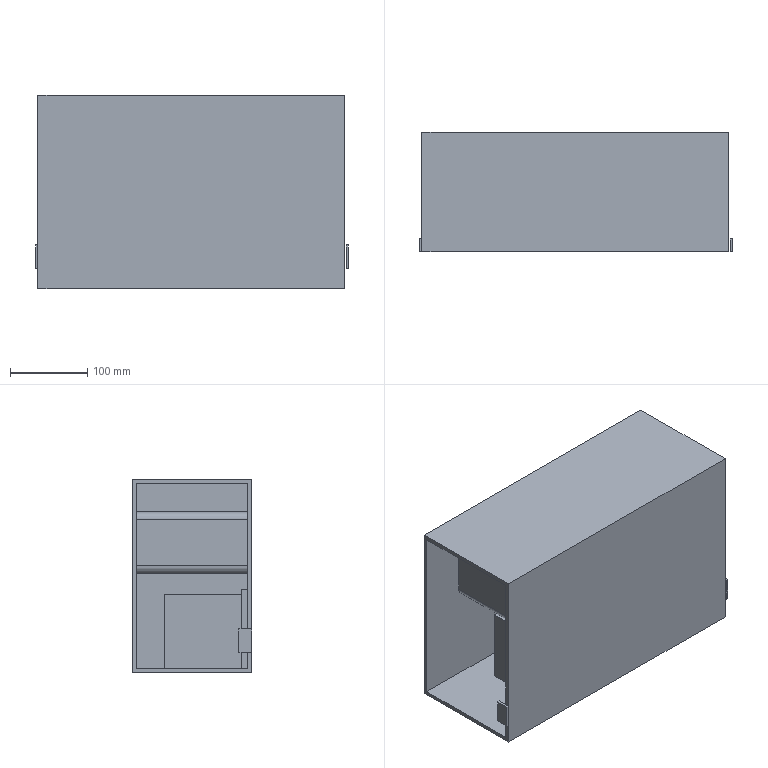Part | SolidWorks | features BaseBody 5 | 5 solids | 51 faces | box 406 x 155 x 251.525 mm | volume 5535552 mm3 | plane 43 | cylinder 8 | commonest cylinder face diameters 20 x8
STEP:
#1=CARTESIAN_POINT('',(141.539,102.72,635.851));
#2=VERTEX_POINT('',#1);
#3=CARTESIAN_POINT('',(271.539,102.72,635.851));
#4=VERTEX_POINT('',#3);
#5=CARTESIAN_POINT('',(0.,102.72,635.851));
#6=DIRECTION('',(1.,0.,0.));
#7=VECTOR('',#6,1000.);
#8=LINE('',#5,#7);
#9=EDGE_CURVE('',#2,#4,#8,.T.);
#10=ORIENTED_EDGE('',*,*,#9,.T.);
#11=CARTESIAN_POINT('',(271.539,102.72,532.815));
#12=VERTEX_POINT('',#11);
#13=CARTESIAN_POINT('',(271.539,102.72,-148.475));
#14=DIRECTION('',(0.,0.,-1.));
#15=VECTOR('',#14,1000.);
#16=LINE('',#13,#15);
#17=EDGE_CURVE('',#4,#12,#16,.T.);
#18=ORIENTED_EDGE('',*,*,#17,.T.);
#19=CARTESIAN_POINT('',(141.539,102.72,532.815));
#20=VERTEX_POINT('',#19);
#21=CARTESIAN_POINT('',(0.,102.72,532.815));
#22=DIRECTION('',(-1.,0.,0.));
#23=VECTOR('',#22,1000.);
#24=LINE('',#21,#23);
#25=EDGE_CURVE('',#12,#20,#24,.T.);
#26=ORIENTED_EDGE('',*,*,#25,.T.);
#27=CARTESIAN_POINT('',(141.539,102.72,-148.475));
#28=DIRECTION('',(0.,0.,1.));
#29=VECTOR('',#28,1000.);
#30=LINE('',#27,#29);
#31=EDGE_CURVE('',#20,#2,#30,.T.);
#32=ORIENTED_EDGE('',*,*,#31,.T.);
#33=EDGE_LOOP('',(#10,#18,#26,#32));
#34=FACE_OUTER_BOUND('',#33,.T.);
#35=CARTESIAN_POINT('',(0.,102.72,-148.475));
#36=DIRECTION('',(0.,1.,0.));
#37=DIRECTION('',(0.,0.,1.));
#38=AXIS2_PLACEMENT_3D('',#35,#36,#37);
#39=PLANE('',#38);
#40=ADVANCED_FACE('',(#34),#39,.T.);
#41=CARTESIAN_POINT('',(271.539,94.72,532.815));
#42=VERTEX_POINT('',#41);
#43=CARTESIAN_POINT('',(271.539,102.72,532.815));
#44=DIRECTION('',(0.,-1.,0.));
#45=VECTOR('',#44,1000.);
#46=LINE('',#43,#45);
#47=EDGE_CURVE('',#12,#42,#46,.T.);
#48=ORIENTED_EDGE('',*,*,#47,.F.);
#49=ORIENTED_EDGE('',*,*,#17,.F.);
#50=CARTESIAN_POINT('',(271.539,94.72,635.851));
#51=VERTEX_POINT('',#50);
#52=CARTESIAN_POINT('',(271.539,102.72,635.851));
#53=DIRECTION('',(0.,1.,0.));
#54=VECTOR('',#53,1000.);
#55=LINE('',#52,#54);
#56=EDGE_CURVE('',#51,#4,#55,.T.);
#57=ORIENTED_EDGE('',*,*,#56,.F.);
#58=CARTESIAN_POINT('',(271.539,94.72,475.851));
#59=DIRECTION('',(0.,0.,1.));
#60=VECTOR('',#59,1000.);
#61=LINE('',#58,#60);
#62=EDGE_CURVE('',#42,#51,#61,.T.);
#63=ORIENTED_EDGE('',*,*,#62,.F.);
#64=EDGE_LOOP('',(#48,#49,#57,#63));
#65=FACE_OUTER_BOUND('',#64,.T.);
#66=CARTESIAN_POINT('',(271.539,102.72,475.851));
#67=DIRECTION('',(-1.,0.,0.));
#68=DIRECTION('',(0.,0.,1.));
#69=AXIS2_PLACEMENT_3D('',#66,#67,#68);
#70=PLANE('',#69);
#71=ADVANCED_FACE('',(#65),#70,.F.);
#72=ORIENTED_EDGE('',*,*,#56,.T.);
#73=ORIENTED_EDGE('',*,*,#9,.F.);
#74=CARTESIAN_POINT('',(141.539,94.72,635.851));
#75=VERTEX_POINT('',#74);
#76=CARTESIAN_POINT('',(141.539,102.72,635.851));
#77=DIRECTION('',(0.,1.,0.));
#78=VECTOR('',#77,1000.);
#79=LINE('',#76,#78);
#80=EDGE_CURVE('',#75,#2,#79,.T.);
#81=ORIENTED_EDGE('',*,*,#80,.F.);
#82=CARTESIAN_POINT('',(141.539,94.72,635.851));
#83=DIRECTION('',(-1.,0.,0.));
#84=VECTOR('',#83,1000.);
#85=LINE('',#82,#84);
#86=EDGE_CURVE('',#51,#75,#85,.T.);
#87=ORIENTED_EDGE('',*,*,#86,.F.);
#88=EDGE_LOOP('',(#72,#73,#81,#87));
#89=FACE_OUTER_BOUND('',#88,.T.);
#90=CARTESIAN_POINT('',(141.539,102.72,635.851));
#91=DIRECTION('',(0.,0.,-1.));
#92=DIRECTION('',(-1.,0.,0.));
#93=AXIS2_PLACEMENT_3D('',#90,#91,#92);
#94=PLANE('',#93);
#95=ADVANCED_FACE('',(#89),#94,.F.);
#96=CARTESIAN_POINT('',(141.539,94.72,532.815));
#97=VERTEX_POINT('',#96);
#98=CARTESIAN_POINT('',(141.539,102.72,532.815));
#99=DIRECTION('',(0.,1.,0.));
#100=VECTOR('',#99,1000.);
#101=LINE('',#98,#100);
#102=EDGE_CURVE('',#97,#20,#101,.T.);
#103=ORIENTED_EDGE('',*,*,#102,.F.);
#104=CARTESIAN_POINT('',(141.539,94.72,475.851));
#105=DIRECTION('',(0.,0.,-1.));
#106=VECTOR('',#105,1000.);
#107=LINE('',#104,#106);
#108=EDGE_CURVE('',#75,#97,#107,.T.);
#109=ORIENTED_EDGE('',*,*,#108,.F.);
#110=ORIENTED_EDGE('',*,*,#80,.T.);
#111=ORIENTED_EDGE('',*,*,#31,.F.);
#112=EDGE_LOOP('',(#103,#109,#110,#111));
#113=FACE_OUTER_BOUND('',#112,.T.);
#114=CARTESIAN_POINT('',(141.539,102.72,475.851));
#115=DIRECTION('',(1.,0.,0.));
#116=DIRECTION('',(0.,0.,-1.));
#117=AXIS2_PLACEMENT_3D('',#114,#115,#116);
#118=PLANE('',#117);
#119=ADVANCED_FACE('',(#113),#118,.F.);
#120=ORIENTED_EDGE('',*,*,#47,.T.);
#121=CARTESIAN_POINT('',(460.124,94.72,532.815));
#122=DIRECTION('',(1.,0.,0.));
#123=VECTOR('',#122,1000.);
#124=LINE('',#121,#123);
#125=EDGE_CURVE('',#97,#42,#124,.T.);
#126=ORIENTED_EDGE('',*,*,#125,.F.);
#127=ORIENTED_EDGE('',*,*,#102,.T.);
#128=ORIENTED_EDGE('',*,*,#25,.F.);
#129=EDGE_LOOP('',(#120,#126,#127,#128));
#130=FACE_OUTER_BOUND('',#129,.T.);
#131=CARTESIAN_POINT('',(460.124,-110.28,532.815));
#132=DIRECTION('',(0.,0.,1.));
#133=DIRECTION('',(1.,0.,0.));
#134=AXIS2_PLACEMENT_3D('',#131,#132,#133);
#135=PLANE('',#134);
#136=ADVANCED_FACE('',(#130),#135,.F.);
#137=ORIENTED_EDGE('',*,*,#125,.T.);
#138=ORIENTED_EDGE('',*,*,#62,.T.);
#139=ORIENTED_EDGE('',*,*,#86,.T.);
#140=ORIENTED_EDGE('',*,*,#108,.T.);
#141=EDGE_LOOP('',(#137,#138,#139,#140));
#142=FACE_OUTER_BOUND('',#141,.T.);
#143=CARTESIAN_POINT('',(0.,94.72,-148.475));
#144=DIRECTION('',(0.,1.,0.));
#145=DIRECTION('',(0.,0.,1.));
#146=AXIS2_PLACEMENT_3D('',#143,#144,#145);
#147=PLANE('',#146);
#148=ADVANCED_FACE('',(#142),#147,.F.);
#149=CLOSED_SHELL('',(#40,#71,#95,#119,#136,#148));
#150=MANIFOLD_SOLID_BREP('',#149);
#151=CARTESIAN_POINT('',(460.124,89.72,584.76));
#152=VERTEX_POINT('',#151);
#153=CARTESIAN_POINT('',(460.124,89.72,554.76));
#154=VERTEX_POINT('',#153);
#155=CARTESIAN_POINT('',(460.124,89.72,584.76));
#156=DIRECTION('',(0.,0.,-1.));
#157=VECTOR('',#156,1000.);
#158=LINE('',#155,#157);
#159=EDGE_CURVE('',#152,#154,#158,.T.);
#160=ORIENTED_EDGE('',*,*,#159,.F.);
#161=CARTESIAN_POINT('',(460.124,106.359,584.76));
#162=VERTEX_POINT('',#161);
#163=CARTESIAN_POINT('',(460.124,72.987,584.76));
#164=DIRECTION('',(0.,-1.,0.));
#165=VECTOR('',#164,1000.);
#166=LINE('',#163,#165);
#167=EDGE_CURVE('',#162,#152,#166,.T.);
#168=ORIENTED_EDGE('',*,*,#167,.F.);
#169=CARTESIAN_POINT('',(460.124,106.359,554.76));
#170=VERTEX_POINT('',#169);
#171=CARTESIAN_POINT('',(460.124,106.359,584.76));
#172=DIRECTION('',(0.,0.,1.));
#173=VECTOR('',#172,1000.);
#174=LINE('',#171,#173);
#175=EDGE_CURVE('',#170,#162,#174,.T.);
#176=ORIENTED_EDGE('',*,*,#175,.F.);
#177=CARTESIAN_POINT('',(460.124,72.987,554.76));
#178=DIRECTION('',(0.,1.,0.));
#179=VECTOR('',#178,1000.);
#180=LINE('',#177,#179);
#181=EDGE_CURVE('',#154,#170,#180,.T.);
#182=ORIENTED_EDGE('',*,*,#181,.F.);
#183=EDGE_LOOP('',(#160,#168,#176,#182));
#184=FACE_OUTER_BOUND('',#183,.T.);
#185=CARTESIAN_POINT('',(460.124,72.987,584.76));
#186=DIRECTION('',(1.,0.,0.));
#187=DIRECTION('',(0.,0.,-1.));
#188=AXIS2_PLACEMENT_3D('',#185,#186,#187);
#189=PLANE('',#188);
#190=ADVANCED_FACE('',(#184),#189,.F.);
#191=CARTESIAN_POINT('',(463.124,106.359,554.76));
#192=VERTEX_POINT('',#191);
#193=CARTESIAN_POINT('',(260.124,106.359,554.76));
#194=DIRECTION('',(1.,0.,0.));
#195=VECTOR('',#194,1000.);
#196=LINE('',#193,#195);
#197=EDGE_CURVE('',#170,#192,#196,.T.);
#198=ORIENTED_EDGE('',*,*,#197,.T.);
#199=CARTESIAN_POINT('',(463.124,89.72,554.76));
#200=VERTEX_POINT('',#199);
#201=CARTESIAN_POINT('',(463.124,59.72,554.76));
#202=DIRECTION('',(0.,-1.,0.));
#203=VECTOR('',#202,1000.);
#204=LINE('',#201,#203);
#205=EDGE_CURVE('',#192,#200,#204,.T.);
#206=ORIENTED_EDGE('',*,*,#205,.T.);
#207=CARTESIAN_POINT('',(260.124,89.72,554.76));
#208=DIRECTION('',(-1.,0.,0.));
#209=VECTOR('',#208,1000.);
#210=LINE('',#207,#209);
#211=EDGE_CURVE('',#200,#154,#210,.T.);
#212=ORIENTED_EDGE('',*,*,#211,.T.);
#213=ORIENTED_EDGE('',*,*,#181,.T.);
#214=EDGE_LOOP('',(#198,#206,#212,#213));
#215=FACE_OUTER_BOUND('',#214,.T.);
#216=CARTESIAN_POINT('',(260.124,59.72,554.76));
#217=DIRECTION('',(0.,0.,-1.));
#218=DIRECTION('',(-1.,0.,0.));
#219=AXIS2_PLACEMENT_3D('',#216,#217,#218);
#220=PLANE('',#219);
#221=ADVANCED_FACE('',(#215),#220,.T.);
#222=ORIENTED_EDGE('',*,*,#211,.F.);
#223=CARTESIAN_POINT('',(463.124,89.72,584.76));
#224=VERTEX_POINT('',#223);
#225=CARTESIAN_POINT('',(463.124,89.72,0.));
#226=DIRECTION('',(0.,0.,-1.));
#227=VECTOR('',#226,1000.);
#228=LINE('',#225,#227);
#229=EDGE_CURVE('',#224,#200,#228,.T.);
#230=ORIENTED_EDGE('',*,*,#229,.F.);
#231=CARTESIAN_POINT('',(0.,89.72,584.76));
#232=DIRECTION('',(1.,0.,0.));
#233=VECTOR('',#232,1000.);
#234=LINE('',#231,#233);
#235=EDGE_CURVE('',#152,#224,#234,.T.);
#236=ORIENTED_EDGE('',*,*,#235,.F.);
#237=ORIENTED_EDGE('',*,*,#159,.T.);
#238=EDGE_LOOP('',(#222,#230,#236,#237));
#239=FACE_OUTER_BOUND('',#238,.T.);
#240=CARTESIAN_POINT('',(0.,89.72,0.));
#241=DIRECTION('',(0.,1.,0.));
#242=DIRECTION('',(0.,0.,1.));
#243=AXIS2_PLACEMENT_3D('',#240,#241,#242);
#244=PLANE('',#243);
#245=ADVANCED_FACE('',(#239),#244,.F.);
#246=ORIENTED_EDGE('',*,*,#235,.T.);
#247=CARTESIAN_POINT('',(463.124,106.359,584.76));
#248=VERTEX_POINT('',#247);
#249=CARTESIAN_POINT('',(463.124,59.72,584.76));
#250=DIRECTION('',(0.,-1.,0.));
#251=VECTOR('',#250,1000.);
#252=LINE('',#249,#251);
#253=EDGE_CURVE('',#248,#224,#252,.T.);
#254=ORIENTED_EDGE('',*,*,#253,.F.);
#255=CARTESIAN_POINT('',(260.124,106.359,584.76));
#256=DIRECTION('',(1.,0.,0.));
#257=VECTOR('',#256,1000.);
#258=LINE('',#255,#257);
#259=EDGE_CURVE('',#162,#248,#258,.T.);
#260=ORIENTED_EDGE('',*,*,#259,.F.);
#261=ORIENTED_EDGE('',*,*,#167,.T.);
#262=EDGE_LOOP('',(#246,#254,#260,#261));
#263=FACE_OUTER_BOUND('',#262,.T.);
#264=CARTESIAN_POINT('',(260.124,59.72,584.76));
#265=DIRECTION('',(0.,0.,-1.));
#266=DIRECTION('',(-1.,0.,0.));
#267=AXIS2_PLACEMENT_3D('',#264,#265,#266);
#268=PLANE('',#267);
#269=ADVANCED_FACE('',(#263),#268,.F.);
#270=ORIENTED_EDGE('',*,*,#175,.T.);
#271=ORIENTED_EDGE('',*,*,#259,.T.);
#272=CARTESIAN_POINT('',(463.124,106.359,584.76));
#273=DIRECTION('',(0.,0.,1.));
#274=VECTOR('',#273,1000.);
#275=LINE('',#272,#274);
#276=EDGE_CURVE('',#192,#248,#275,.T.);
#277=ORIENTED_EDGE('',*,*,#276,.F.);
#278=ORIENTED_EDGE('',*,*,#197,.F.);
#279=EDGE_LOOP('',(#270,#271,#277,#278));
#280=FACE_OUTER_BOUND('',#279,.T.);
#281=CARTESIAN_POINT('',(463.124,106.359,584.76));
#282=DIRECTION('',(0.,-1.,0.));
#283=DIRECTION('',(0.,0.,-1.));
#284=AXIS2_PLACEMENT_3D('',#281,#282,#283);
#285=PLANE('',#284);
#286=ADVANCED_FACE('',(#280),#285,.F.);
#287=ORIENTED_EDGE('',*,*,#229,.T.);
#288=ORIENTED_EDGE('',*,*,#205,.F.);
#289=ORIENTED_EDGE('',*,*,#276,.T.);
#290=ORIENTED_EDGE('',*,*,#253,.T.);
#291=EDGE_LOOP('',(#287,#288,#289,#290));
#292=FACE_OUTER_BOUND('',#291,.T.);
#293=CARTESIAN_POINT('',(463.124,72.987,584.76));
#294=DIRECTION('',(-1.,0.,0.));
#295=DIRECTION('',(0.,0.,1.));
#296=AXIS2_PLACEMENT_3D('',#293,#294,#295);
#297=PLANE('',#296);
#298=ADVANCED_FACE('',(#292),#297,.F.);
#299=CLOSED_SHELL('',(#190,#221,#245,#269,#286,#298));
#300=MANIFOLD_SOLID_BREP('',#299);
#301=CARTESIAN_POINT('',(265.539,102.72,532.815));
#302=VERTEX_POINT('',#301);
#303=CARTESIAN_POINT('',(265.539,202.72,532.815));
#304=VERTEX_POINT('',#303);
#305=CARTESIAN_POINT('',(265.539,-110.28,532.815));
#306=DIRECTION('',(0.,1.,0.));
#307=VECTOR('',#306,1000.);
#308=LINE('',#305,#307);
#309=EDGE_CURVE('',#302,#304,#308,.T.);
#310=ORIENTED_EDGE('',*,*,#309,.F.);
#311=CARTESIAN_POINT('',(147.539,102.72,532.815));
#312=VERTEX_POINT('',#311);
#313=CARTESIAN_POINT('',(460.124,102.72,532.815));
#314=DIRECTION('',(1.,0.,0.));
#315=VECTOR('',#314,1000.);
#316=LINE('',#313,#315);
#317=EDGE_CURVE('',#312,#302,#316,.T.);
#318=ORIENTED_EDGE('',*,*,#317,.F.);
#319=CARTESIAN_POINT('',(147.539,202.72,532.815));
#320=VERTEX_POINT('',#319);
#321=CARTESIAN_POINT('',(147.539,-110.28,532.815));
#322=DIRECTION('',(0.,-1.,0.));
#323=VECTOR('',#322,1000.);
#324=LINE('',#321,#323);
#325=EDGE_CURVE('',#320,#312,#324,.T.);
#326=ORIENTED_EDGE('',*,*,#325,.F.);
#327=CARTESIAN_POINT('',(460.124,202.72,532.815));
#328=DIRECTION('',(-1.,0.,0.));
#329=VECTOR('',#328,1000.);
#330=LINE('',#327,#329);
#331=EDGE_CURVE('',#304,#320,#330,.T.);
#332=ORIENTED_EDGE('',*,*,#331,.F.);
#333=EDGE_LOOP('',(#310,#318,#326,#332));
#334=FACE_OUTER_BOUND('',#333,.T.);
#335=CARTESIAN_POINT('',(460.124,-110.28,532.815));
#336=DIRECTION('',(0.,0.,1.));
#337=DIRECTION('',(1.,0.,0.));
#338=AXIS2_PLACEMENT_3D('',#335,#336,#337);
#339=PLANE('',#338);
#340=ADVANCED_FACE('',(#334),#339,.F.);
#341=CARTESIAN_POINT('',(147.539,202.72,629.851));
#342=VERTEX_POINT('',#341);
#343=CARTESIAN_POINT('',(265.539,202.72,629.851));
#344=VERTEX_POINT('',#343);
#345=CARTESIAN_POINT('',(0.,202.72,629.851));
#346=DIRECTION('',(1.,0.,0.));
#347=VECTOR('',#346,1000.);
#348=LINE('',#345,#347);
#349=EDGE_CURVE('',#342,#344,#348,.T.);
#350=ORIENTED_EDGE('',*,*,#349,.T.);
#351=CARTESIAN_POINT('',(265.539,202.72,-148.475));
#352=DIRECTION('',(0.,0.,-1.));
#353=VECTOR('',#352,1000.);
#354=LINE('',#351,#353);
#355=EDGE_CURVE('',#344,#304,#354,.T.);
#356=ORIENTED_EDGE('',*,*,#355,.T.);
#357=ORIENTED_EDGE('',*,*,#331,.T.);
#358=CARTESIAN_POINT('',(147.539,202.72,-148.475));
#359=DIRECTION('',(0.,0.,1.));
#360=VECTOR('',#359,1000.);
#361=LINE('',#358,#360);
#362=EDGE_CURVE('',#320,#342,#361,.T.);
#363=ORIENTED_EDGE('',*,*,#362,.T.);
#364=EDGE_LOOP('',(#350,#356,#357,#363));
#365=FACE_OUTER_BOUND('',#364,.T.);
#366=CARTESIAN_POINT('',(0.,202.72,-148.475));
#367=DIRECTION('',(0.,1.,0.));
#368=DIRECTION('',(0.,0.,1.));
#369=AXIS2_PLACEMENT_3D('',#366,#367,#368);
#370=PLANE('',#369);
#371=ADVANCED_FACE('',(#365),#370,.T.);
#372=ORIENTED_EDGE('',*,*,#309,.T.);
#373=ORIENTED_EDGE('',*,*,#355,.F.);
#374=CARTESIAN_POINT('',(265.539,102.72,629.851));
#375=VERTEX_POINT('',#374);
#376=CARTESIAN_POINT('',(265.539,202.72,629.851));
#377=DIRECTION('',(0.,1.,0.));
#378=VECTOR('',#377,1000.);
#379=LINE('',#376,#378);
#380=EDGE_CURVE('',#375,#344,#379,.T.);
#381=ORIENTED_EDGE('',*,*,#380,.F.);
#382=CARTESIAN_POINT('',(265.539,102.72,629.851));
#383=DIRECTION('',(0.,0.,1.));
#384=VECTOR('',#383,1000.);
#385=LINE('',#382,#384);
#386=EDGE_CURVE('',#302,#375,#385,.T.);
#387=ORIENTED_EDGE('',*,*,#386,.F.);
#388=EDGE_LOOP('',(#372,#373,#381,#387));
#389=FACE_OUTER_BOUND('',#388,.T.);
#390=CARTESIAN_POINT('',(265.539,202.72,629.851));
#391=DIRECTION('',(-1.,0.,0.));
#392=DIRECTION('',(0.,0.,1.));
#393=AXIS2_PLACEMENT_3D('',#390,#391,#392);
#394=PLANE('',#393);
#395=ADVANCED_FACE('',(#389),#394,.F.);
#396=ORIENTED_EDGE('',*,*,#317,.T.);
#397=ORIENTED_EDGE('',*,*,#386,.T.);
#398=CARTESIAN_POINT('',(147.539,102.72,629.851));
#399=VERTEX_POINT('',#398);
#400=CARTESIAN_POINT('',(0.,102.72,629.851));
#401=DIRECTION('',(1.,0.,0.));
#402=VECTOR('',#401,1000.);
#403=LINE('',#400,#402);
#404=EDGE_CURVE('',#399,#375,#403,.T.);
#405=ORIENTED_EDGE('',*,*,#404,.F.);
#406=CARTESIAN_POINT('',(147.539,102.72,-148.475));
#407=DIRECTION('',(0.,0.,1.));
#408=VECTOR('',#407,1000.);
#409=LINE('',#406,#408);
#410=EDGE_CURVE('',#312,#399,#409,.T.);
#411=ORIENTED_EDGE('',*,*,#410,.F.);
#412=EDGE_LOOP('',(#396,#397,#405,#411));
#413=FACE_OUTER_BOUND('',#412,.T.);
#414=CARTESIAN_POINT('',(0.,102.72,-148.475));
#415=DIRECTION('',(0.,1.,0.));
#416=DIRECTION('',(0.,0.,1.));
#417=AXIS2_PLACEMENT_3D('',#414,#415,#416);
#418=PLANE('',#417);
#419=ADVANCED_FACE('',(#413),#418,.F.);
#420=ORIENTED_EDGE('',*,*,#325,.T.);
#421=ORIENTED_EDGE('',*,*,#410,.T.);
#422=CARTESIAN_POINT('',(147.539,202.72,629.851));
#423=DIRECTION('',(0.,-1.,0.));
#424=VECTOR('',#423,1000.);
#425=LINE('',#422,#424);
#426=EDGE_CURVE('',#342,#399,#425,.T.);
#427=ORIENTED_EDGE('',*,*,#426,.F.);
#428=ORIENTED_EDGE('',*,*,#362,.F.);
#429=EDGE_LOOP('',(#420,#421,#427,#428));
#430=FACE_OUTER_BOUND('',#429,.T.);
#431=CARTESIAN_POINT('',(147.539,202.72,481.851));
#432=DIRECTION('',(1.,0.,0.));
#433=DIRECTION('',(0.,0.,-1.));
#434=AXIS2_PLACEMENT_3D('',#431,#432,#433);
#435=PLANE('',#434);
#436=ADVANCED_FACE('',(#430),#435,.F.);
#437=ORIENTED_EDGE('',*,*,#380,.T.);
#438=ORIENTED_EDGE('',*,*,#349,.F.);
#439=ORIENTED_EDGE('',*,*,#426,.T.);
#440=ORIENTED_EDGE('',*,*,#404,.T.);
#441=EDGE_LOOP('',(#437,#438,#439,#440));
#442=FACE_OUTER_BOUND('',#441,.T.);
#443=CARTESIAN_POINT('',(147.539,202.72,629.851));
#444=DIRECTION('',(0.,0.,-1.));
#445=DIRECTION('',(-1.,0.,0.));
#446=AXIS2_PLACEMENT_3D('',#443,#444,#445);
#447=PLANE('',#446);
#448=ADVANCED_FACE('',(#442),#447,.F.);
#449=CLOSED_SHELL('',(#340,#371,#395,#419,#436,#448));
#450=MANIFOLD_SOLID_BREP('',#449);
#451=CARTESIAN_POINT('',(60.124,89.72,554.76));
#452=VERTEX_POINT('',#451);
#453=CARTESIAN_POINT('',(60.124,89.72,584.76));
#454=VERTEX_POINT('',#453);
#455=CARTESIAN_POINT('',(60.124,89.72,584.76));
#456=DIRECTION('',(0.,0.,1.));
#457=VECTOR('',#456,1000.);
#458=LINE('',#455,#457);
#459=EDGE_CURVE('',#452,#454,#458,.T.);
#460=ORIENTED_EDGE('',*,*,#459,.F.);
#461=CARTESIAN_POINT('',(60.124,106.359,554.76));
#462=VERTEX_POINT('',#461);
#463=CARTESIAN_POINT('',(60.124,72.987,554.76));
#464=DIRECTION('',(0.,-1.,0.));
#465=VECTOR('',#464,1000.);
#466=LINE('',#463,#465);
#467=EDGE_CURVE('',#462,#452,#466,.T.);
#468=ORIENTED_EDGE('',*,*,#467,.F.);
#469=CARTESIAN_POINT('',(60.124,106.359,584.76));
#470=VERTEX_POINT('',#469);
#471=CARTESIAN_POINT('',(60.124,106.359,584.76));
#472=DIRECTION('',(0.,0.,-1.));
#473=VECTOR('',#472,1000.);
#474=LINE('',#471,#473);
#475=EDGE_CURVE('',#470,#462,#474,.T.);
#476=ORIENTED_EDGE('',*,*,#475,.F.);
#477=CARTESIAN_POINT('',(60.124,72.987,584.76));
#478=DIRECTION('',(0.,1.,0.));
#479=VECTOR('',#478,1000.);
#480=LINE('',#477,#479);
#481=EDGE_CURVE('',#454,#470,#480,.T.);
#482=ORIENTED_EDGE('',*,*,#481,.F.);
#483=EDGE_LOOP('',(#460,#468,#476,#482));
#484=FACE_OUTER_BOUND('',#483,.T.);
#485=CARTESIAN_POINT('',(60.124,72.987,584.76));
#486=DIRECTION('',(-1.,0.,0.));
#487=DIRECTION('',(0.,0.,1.));
#488=AXIS2_PLACEMENT_3D('',#485,#486,#487);
#489=PLANE('',#488);
#490=ADVANCED_FACE('',(#484),#489,.F.);
#491=CARTESIAN_POINT('',(57.124,89.72,584.76));
#492=VERTEX_POINT('',#491);
#493=CARTESIAN_POINT('',(260.124,89.72,584.76));
#494=DIRECTION('',(-1.,0.,0.));
#495=VECTOR('',#494,1000.);
#496=LINE('',#493,#495);
#497=EDGE_CURVE('',#454,#492,#496,.T.);
#498=ORIENTED_EDGE('',*,*,#497,.F.);
#499=ORIENTED_EDGE('',*,*,#481,.T.);
#500=CARTESIAN_POINT('',(57.124,106.359,584.76));
#501=VERTEX_POINT('',#500);
#502=CARTESIAN_POINT('',(260.124,106.359,584.76));
#503=DIRECTION('',(1.,0.,0.));
#504=VECTOR('',#503,1000.);
#505=LINE('',#502,#504);
#506=EDGE_CURVE('',#501,#470,#505,.T.);
#507=ORIENTED_EDGE('',*,*,#506,.F.);
#508=CARTESIAN_POINT('',(57.124,59.72,584.76));
#509=DIRECTION('',(0.,1.,0.));
#510=VECTOR('',#509,1000.);
#511=LINE('',#508,#510);
#512=EDGE_CURVE('',#492,#501,#511,.T.);
#513=ORIENTED_EDGE('',*,*,#512,.F.);
#514=EDGE_LOOP('',(#498,#499,#507,#513));
#515=FACE_OUTER_BOUND('',#514,.T.);
#516=CARTESIAN_POINT('',(260.124,59.72,584.76));
#517=DIRECTION('',(0.,0.,-1.));
#518=DIRECTION('',(-1.,0.,0.));
#519=AXIS2_PLACEMENT_3D('',#516,#517,#518);
#520=PLANE('',#519);
#521=ADVANCED_FACE('',(#515),#520,.F.);
#522=CARTESIAN_POINT('',(57.124,89.72,554.76));
#523=VERTEX_POINT('',#522);
#524=CARTESIAN_POINT('',(0.,89.72,554.76));
#525=DIRECTION('',(-1.,0.,0.));
#526=VECTOR('',#525,1000.);
#527=LINE('',#524,#526);
#528=EDGE_CURVE('',#452,#523,#527,.T.);
#529=ORIENTED_EDGE('',*,*,#528,.F.);
#530=ORIENTED_EDGE('',*,*,#459,.T.);
#531=ORIENTED_EDGE('',*,*,#497,.T.);
#532=CARTESIAN_POINT('',(57.124,89.72,0.));
#533=DIRECTION('',(0.,0.,1.));
#534=VECTOR('',#533,1000.);
#535=LINE('',#532,#534);
#536=EDGE_CURVE('',#523,#492,#535,.T.);
#537=ORIENTED_EDGE('',*,*,#536,.F.);
#538=EDGE_LOOP('',(#529,#530,#531,#537));
#539=FACE_OUTER_BOUND('',#538,.T.);
#540=CARTESIAN_POINT('',(0.,89.72,0.));
#541=DIRECTION('',(0.,1.,0.));
#542=DIRECTION('',(0.,0.,1.));
#543=AXIS2_PLACEMENT_3D('',#540,#541,#542);
#544=PLANE('',#543);
#545=ADVANCED_FACE('',(#539),#544,.F.);
#546=CARTESIAN_POINT('',(57.124,106.359,554.76));
#547=VERTEX_POINT('',#546);
#548=CARTESIAN_POINT('',(260.124,106.359,554.76));
#549=DIRECTION('',(1.,0.,0.));
#550=VECTOR('',#549,1000.);
#551=LINE('',#548,#550);
#552=EDGE_CURVE('',#547,#462,#551,.T.);
#553=ORIENTED_EDGE('',*,*,#552,.T.);
#554=ORIENTED_EDGE('',*,*,#467,.T.);
#555=ORIENTED_EDGE('',*,*,#528,.T.);
#556=CARTESIAN_POINT('',(57.124,59.72,554.76));
#557=DIRECTION('',(0.,1.,0.));
#558=VECTOR('',#557,1000.);
#559=LINE('',#556,#558);
#560=EDGE_CURVE('',#523,#547,#559,.T.);
#561=ORIENTED_EDGE('',*,*,#560,.T.);
#562=EDGE_LOOP('',(#553,#554,#555,#561));
#563=FACE_OUTER_BOUND('',#562,.T.);
#564=CARTESIAN_POINT('',(260.124,59.72,554.76));
#565=DIRECTION('',(0.,0.,-1.));
#566=DIRECTION('',(-1.,0.,0.));
#567=AXIS2_PLACEMENT_3D('',#564,#565,#566);
#568=PLANE('',#567);
#569=ADVANCED_FACE('',(#563),#568,.T.);
#570=CARTESIAN_POINT('',(57.124,106.359,584.76));
#571=DIRECTION('',(0.,0.,-1.));
#572=VECTOR('',#571,1000.);
#573=LINE('',#570,#572);
#574=EDGE_CURVE('',#501,#547,#573,.T.);
#575=ORIENTED_EDGE('',*,*,#574,.F.);
#576=ORIENTED_EDGE('',*,*,#506,.T.);
#577=ORIENTED_EDGE('',*,*,#475,.T.);
#578=ORIENTED_EDGE('',*,*,#552,.F.);
#579=EDGE_LOOP('',(#575,#576,#577,#578));
#580=FACE_OUTER_BOUND('',#579,.T.);
#581=CARTESIAN_POINT('',(57.124,106.359,584.76));
#582=DIRECTION('',(0.,-1.,0.));
#583=DIRECTION('',(0.,0.,-1.));
#584=AXIS2_PLACEMENT_3D('',#581,#582,#583);
#585=PLANE('',#584);
#586=ADVANCED_FACE('',(#580),#585,.F.);
#587=ORIENTED_EDGE('',*,*,#536,.T.);
#588=ORIENTED_EDGE('',*,*,#512,.T.);
#589=ORIENTED_EDGE('',*,*,#574,.T.);
#590=ORIENTED_EDGE('',*,*,#560,.F.);
#591=EDGE_LOOP('',(#587,#588,#589,#590));
#592=FACE_OUTER_BOUND('',#591,.T.);
#593=CARTESIAN_POINT('',(57.124,72.987,584.76));
#594=DIRECTION('',(1.,0.,0.));
#595=DIRECTION('',(0.,0.,-1.));
#596=AXIS2_PLACEMENT_3D('',#593,#594,#595);
#597=PLANE('',#596);
#598=ADVANCED_FACE('',(#592),#597,.F.);
#599=CLOSED_SHELL('',(#490,#521,#545,#569,#586,#598));
#600=MANIFOLD_SOLID_BREP('',#599);
#601=CARTESIAN_POINT('',(60.124,89.72,779.34));
#602=VERTEX_POINT('',#601);
#603=CARTESIAN_POINT('',(458.124,89.72,779.34));
#604=VERTEX_POINT('',#603);
#605=CARTESIAN_POINT('',(0.,89.72,779.34));
#606=DIRECTION('',(1.,0.,0.));
#607=VECTOR('',#606,1000.);
#608=LINE('',#605,#607);
#609=EDGE_CURVE('',#602,#604,#608,.T.);
#610=ORIENTED_EDGE('',*,*,#609,.F.);
#611=CARTESIAN_POINT('',(60.124,89.72,527.815));
#612=VERTEX_POINT('',#611);
#613=CARTESIAN_POINT('',(60.124,89.72,0.));
#614=DIRECTION('',(0.,0.,1.));
#615=VECTOR('',#614,1000.);
#616=LINE('',#613,#615);
#617=EDGE_CURVE('',#612,#602,#616,.T.);
#618=ORIENTED_EDGE('',*,*,#617,.F.);
#619=CARTESIAN_POINT('',(458.124,89.72,527.815));
#620=VERTEX_POINT('',#619);
#621=CARTESIAN_POINT('',(0.,89.72,527.815));
#622=DIRECTION('',(-1.,0.,0.));
#623=VECTOR('',#622,1000.);
#624=LINE('',#621,#623);
#625=EDGE_CURVE('',#620,#612,#624,.T.);
#626=ORIENTED_EDGE('',*,*,#625,.F.);
#627=CARTESIAN_POINT('',(458.124,89.72,0.));
#628=DIRECTION('',(0.,0.,-1.));
#629=VECTOR('',#628,1000.);
#630=LINE('',#627,#629);
#631=EDGE_CURVE('',#604,#620,#630,.T.);
#632=ORIENTED_EDGE('',*,*,#631,.F.);
#633=EDGE_LOOP('',(#610,#618,#626,#632));
#634=FACE_OUTER_BOUND('',#633,.T.);
#635=CARTESIAN_POINT('',(0.,89.72,0.));
#636=DIRECTION('',(0.,1.,0.));
#637=DIRECTION('',(0.,0.,1.));
#638=AXIS2_PLACEMENT_3D('',#635,#636,#637);
#639=PLANE('',#638);
#640=ADVANCED_FACE('',(#634),#639,.F.);
#641=ORIENTED_EDGE('',*,*,#631,.T.);
#642=CARTESIAN_POINT('',(458.124,244.72,527.815));
#643=VERTEX_POINT('',#642);
#644=CARTESIAN_POINT('',(458.124,389.72,527.815));
#645=DIRECTION('',(0.,-1.,0.));
#646=VECTOR('',#645,1000.);
#647=LINE('',#644,#646);
#648=EDGE_CURVE('',#643,#620,#647,.T.);
#649=ORIENTED_EDGE('',*,*,#648,.F.);
#650=CARTESIAN_POINT('',(458.124,244.72,779.34));
#651=VERTEX_POINT('',#650);
#652=CARTESIAN_POINT('',(458.124,244.72,527.815));
#653=DIRECTION('',(0.,0.,-1.));
#654=VECTOR('',#653,1000.);
#655=LINE('',#652,#654);
#656=EDGE_CURVE('',#651,#643,#655,.T.);
#657=ORIENTED_EDGE('',*,*,#656,.F.);
#658=CARTESIAN_POINT('',(458.124,389.72,779.34));
#659=DIRECTION('',(0.,1.,0.));
#660=VECTOR('',#659,1000.);
#661=LINE('',#658,#660);
#662=EDGE_CURVE('',#604,#651,#661,.T.);
#663=ORIENTED_EDGE('',*,*,#662,.F.);
#664=EDGE_LOOP('',(#641,#649,#657,#663));
#665=FACE_OUTER_BOUND('',#664,.T.);
#666=CARTESIAN_POINT('',(458.124,389.72,527.815));
#667=DIRECTION('',(-1.,0.,0.));
#668=DIRECTION('',(0.,0.,1.));
#669=AXIS2_PLACEMENT_3D('',#666,#667,#668);
#670=PLANE('',#669);
#671=ADVANCED_FACE('',(#665),#670,.F.);
#672=ORIENTED_EDGE('',*,*,#609,.T.);
#673=ORIENTED_EDGE('',*,*,#662,.T.);
#674=CARTESIAN_POINT('',(60.124,244.72,779.34));
#675=VERTEX_POINT('',#674);
#676=CARTESIAN_POINT('',(60.124,244.72,779.34));
#677=DIRECTION('',(1.,0.,0.));
#678=VECTOR('',#677,1000.);
#679=LINE('',#676,#678);
#680=EDGE_CURVE('',#675,#651,#679,.T.);
#681=ORIENTED_EDGE('',*,*,#680,.F.);
#682=CARTESIAN_POINT('',(60.124,244.72,779.34));
#683=DIRECTION('',(0.,1.,0.));
#684=VECTOR('',#683,1000.);
#685=LINE('',#682,#684);
#686=EDGE_CURVE('',#602,#675,#685,.T.);
#687=ORIENTED_EDGE('',*,*,#686,.F.);
#688=EDGE_LOOP('',(#672,#673,#681,#687));
#689=FACE_OUTER_BOUND('',#688,.T.);
#690=CARTESIAN_POINT('',(60.124,244.72,779.34));
#691=DIRECTION('',(0.,0.,-1.));
#692=DIRECTION('',(-1.,0.,0.));
#693=AXIS2_PLACEMENT_3D('',#690,#691,#692);
#694=PLANE('',#693);
#695=ADVANCED_FACE('',(#689),#694,.F.);
#696=CARTESIAN_POINT('',(60.124,239.72,774.34));
#697=VERTEX_POINT('',#696);
#698=CARTESIAN_POINT('',(60.124,239.72,532.815));
#699=VERTEX_POINT('',#698);
#700=CARTESIAN_POINT('',(60.124,239.72,527.815));
#701=DIRECTION('',(0.,0.,-1.));
#702=VECTOR('',#701,1000.);
#703=LINE('',#700,#702);
#704=EDGE_CURVE('',#697,#699,#703,.T.);
#705=ORIENTED_EDGE('',*,*,#704,.F.);
#706=CARTESIAN_POINT('',(60.124,94.72,774.34));
#707=VERTEX_POINT('',#706);
#708=CARTESIAN_POINT('',(60.124,389.72,774.34));
#709=DIRECTION('',(0.,1.,0.));
#710=VECTOR('',#709,1000.);
#711=LINE('',#708,#710);
#712=EDGE_CURVE('',#707,#697,#711,.T.);
#713=ORIENTED_EDGE('',*,*,#712,.F.);
#714=CARTESIAN_POINT('',(60.124,94.72,532.815));
#715=VERTEX_POINT('',#714);
#716=CARTESIAN_POINT('',(60.124,94.72,527.815));
#717=DIRECTION('',(0.,0.,1.));
#718=VECTOR('',#717,1000.);
#719=LINE('',#716,#718);
#720=EDGE_CURVE('',#715,#707,#719,.T.);
#721=ORIENTED_EDGE('',*,*,#720,.F.);
#722=CARTESIAN_POINT('',(60.124,389.72,532.815));
#723=DIRECTION('',(0.,-1.,0.));
#724=VECTOR('',#723,1000.);
#725=LINE('',#722,#724);
#726=EDGE_CURVE('',#699,#715,#725,.T.);
#727=ORIENTED_EDGE('',*,*,#726,.F.);
#728=EDGE_LOOP('',(#705,#713,#721,#727));
#729=FACE_BOUND('',#728,.T.);
#730=ORIENTED_EDGE('',*,*,#686,.T.);
#731=CARTESIAN_POINT('',(60.124,244.72,527.815));
#732=VERTEX_POINT('',#731);
#733=CARTESIAN_POINT('',(60.124,244.72,527.815));
#734=DIRECTION('',(0.,0.,1.));
#735=VECTOR('',#734,1000.);
#736=LINE('',#733,#735);
#737=EDGE_CURVE('',#732,#675,#736,.T.);
#738=ORIENTED_EDGE('',*,*,#737,.F.);
#739=CARTESIAN_POINT('',(60.124,389.72,527.815));
#740=DIRECTION('',(0.,1.,0.));
#741=VECTOR('',#740,1000.);
#742=LINE('',#739,#741);
#743=EDGE_CURVE('',#612,#732,#742,.T.);
#744=ORIENTED_EDGE('',*,*,#743,.F.);
#745=ORIENTED_EDGE('',*,*,#617,.T.);
#746=EDGE_LOOP('',(#730,#738,#744,#745));
#747=FACE_OUTER_BOUND('',#746,.T.);
#748=CARTESIAN_POINT('',(60.124,389.72,527.815));
#749=DIRECTION('',(1.,0.,0.));
#750=DIRECTION('',(0.,0.,-1.));
#751=AXIS2_PLACEMENT_3D('',#748,#749,#750);
#752=PLANE('',#751);
#753=ADVANCED_FACE('',(#729,#747),#752,.F.);
#754=CARTESIAN_POINT('',(60.124,244.72,527.815));
#755=DIRECTION('',(-1.,0.,0.));
#756=VECTOR('',#755,1000.);
#757=LINE('',#754,#756);
#758=EDGE_CURVE('',#643,#732,#757,.T.);
#759=ORIENTED_EDGE('',*,*,#758,.F.);
#760=ORIENTED_EDGE('',*,*,#648,.T.);
#761=ORIENTED_EDGE('',*,*,#625,.T.);
#762=ORIENTED_EDGE('',*,*,#743,.T.);
#763=EDGE_LOOP('',(#759,#760,#761,#762));
#764=FACE_OUTER_BOUND('',#763,.T.);
#765=CARTESIAN_POINT('',(60.124,389.72,527.815));
#766=DIRECTION('',(0.,0.,1.));
#767=DIRECTION('',(1.,0.,0.));
#768=AXIS2_PLACEMENT_3D('',#765,#766,#767);
#769=PLANE('',#768);
#770=ADVANCED_FACE('',(#764),#769,.F.);
#771=ORIENTED_EDGE('',*,*,#656,.T.);
#772=ORIENTED_EDGE('',*,*,#758,.T.);
#773=ORIENTED_EDGE('',*,*,#737,.T.);
#774=ORIENTED_EDGE('',*,*,#680,.T.);
#775=EDGE_LOOP('',(#771,#772,#773,#774));
#776=FACE_OUTER_BOUND('',#775,.T.);
#777=CARTESIAN_POINT('',(0.,244.72,0.));
#778=DIRECTION('',(0.,1.,0.));
#779=DIRECTION('',(0.,0.,1.));
#780=AXIS2_PLACEMENT_3D('',#777,#778,#779);
#781=PLANE('',#780);
#782=ADVANCED_FACE('',(#776),#781,.T.);
#783=ORIENTED_EDGE('',*,*,#726,.T.);
#784=CARTESIAN_POINT('',(453.124,94.72,532.815));
#785=VERTEX_POINT('',#784);
#786=CARTESIAN_POINT('',(60.124,94.72,532.815));
#787=DIRECTION('',(1.,0.,0.));
#788=VECTOR('',#787,1000.);
#789=LINE('',#786,#788);
#790=EDGE_CURVE('',#715,#785,#789,.T.);
#791=ORIENTED_EDGE('',*,*,#790,.T.);
#792=CARTESIAN_POINT('',(453.124,239.72,532.815));
#793=VERTEX_POINT('',#792);
#794=CARTESIAN_POINT('',(453.124,389.72,532.815));
#795=DIRECTION('',(0.,1.,0.));
#796=VECTOR('',#795,1000.);
#797=LINE('',#794,#796);
#798=EDGE_CURVE('',#785,#793,#797,.T.);
#799=ORIENTED_EDGE('',*,*,#798,.T.);
#800=CARTESIAN_POINT('',(60.124,239.72,532.815));
#801=DIRECTION('',(-1.,0.,0.));
#802=VECTOR('',#801,1000.);
#803=LINE('',#800,#802);
#804=EDGE_CURVE('',#793,#699,#803,.T.);
#805=ORIENTED_EDGE('',*,*,#804,.T.);
#806=EDGE_LOOP('',(#783,#791,#799,#805));
#807=FACE_OUTER_BOUND('',#806,.T.);
#808=CARTESIAN_POINT('',(60.124,389.72,532.815));
#809=DIRECTION('',(0.,0.,1.));
#810=DIRECTION('',(1.,0.,0.));
#811=AXIS2_PLACEMENT_3D('',#808,#809,#810);
#812=PLANE('',#811);
#813=ADVANCED_FACE('',(#807),#812,.T.);
#814=CARTESIAN_POINT('',(453.124,239.72,774.34));
#815=VERTEX_POINT('',#814);
#816=CARTESIAN_POINT('',(0.,239.72,774.34));
#817=DIRECTION('',(1.,0.,0.));
#818=VECTOR('',#817,1000.);
#819=LINE('',#816,#818);
#820=EDGE_CURVE('',#697,#815,#819,.T.);
#821=ORIENTED_EDGE('',*,*,#820,.F.);
#822=ORIENTED_EDGE('',*,*,#704,.T.);
#823=ORIENTED_EDGE('',*,*,#804,.F.);
#824=CARTESIAN_POINT('',(453.124,239.72,0.));
#825=DIRECTION('',(0.,0.,-1.));
#826=VECTOR('',#825,1000.);
#827=LINE('',#824,#826);
#828=EDGE_CURVE('',#815,#793,#827,.T.);
#829=ORIENTED_EDGE('',*,*,#828,.F.);
#830=EDGE_LOOP('',(#821,#822,#823,#829));
#831=FACE_OUTER_BOUND('',#830,.T.);
#832=CARTESIAN_POINT('',(228.626,239.72,726.798));
#833=VERTEX_POINT('',#832);
#834=CARTESIAN_POINT('',(218.626,239.72,736.798));
#835=VERTEX_POINT('',#834);
#836=CARTESIAN_POINT('',(218.626,239.72,726.798));
#837=DIRECTION('',(0.,-1.,0.));
#838=DIRECTION('',(0.,0.,-1.));
#839=AXIS2_PLACEMENT_3D('',#836,#837,#838);
#840=CIRCLE('',#839,10.);
#841=EDGE_CURVE('',#833,#835,#840,.T.);
#842=ORIENTED_EDGE('',*,*,#841,.F.);
#843=CARTESIAN_POINT('',(228.626,239.72,666.798));
#844=VERTEX_POINT('',#843);
#845=CARTESIAN_POINT('',(228.626,239.72,0.));
#846=DIRECTION('',(0.,0.,1.));
#847=VECTOR('',#846,1000.);
#848=LINE('',#845,#847);
#849=EDGE_CURVE('',#844,#833,#848,.T.);
#850=ORIENTED_EDGE('',*,*,#849,.F.);
#851=CARTESIAN_POINT('',(218.626,239.72,656.798));
#852=VERTEX_POINT('',#851);
#853=CARTESIAN_POINT('',(218.626,239.72,666.798));
#854=DIRECTION('',(0.,-1.,0.));
#855=DIRECTION('',(0.,0.,-1.));
#856=AXIS2_PLACEMENT_3D('',#853,#854,#855);
#857=CIRCLE('',#856,10.);
#858=EDGE_CURVE('',#852,#844,#857,.T.);
#859=ORIENTED_EDGE('',*,*,#858,.F.);
#860=CARTESIAN_POINT('',(128.626,239.72,656.798));
#861=VERTEX_POINT('',#860);
#862=CARTESIAN_POINT('',(0.,239.72,656.798));
#863=DIRECTION('',(1.,0.,0.));
#864=VECTOR('',#863,1000.);
#865=LINE('',#862,#864);
#866=EDGE_CURVE('',#861,#852,#865,.T.);
#867=ORIENTED_EDGE('',*,*,#866,.F.);
#868=CARTESIAN_POINT('',(118.626,239.72,666.798));
#869=VERTEX_POINT('',#868);
#870=CARTESIAN_POINT('',(128.626,239.72,666.798));
#871=DIRECTION('',(0.,-1.,0.));
#872=DIRECTION('',(0.,0.,-1.));
#873=AXIS2_PLACEMENT_3D('',#870,#871,#872);
#874=CIRCLE('',#873,10.);
#875=EDGE_CURVE('',#869,#861,#874,.T.);
#876=ORIENTED_EDGE('',*,*,#875,.F.);
#877=CARTESIAN_POINT('',(118.626,239.72,726.798));
#878=VERTEX_POINT('',#877);
#879=CARTESIAN_POINT('',(118.626,239.72,0.));
#880=DIRECTION('',(0.,0.,-1.));
#881=VECTOR('',#880,1000.);
#882=LINE('',#879,#881);
#883=EDGE_CURVE('',#878,#869,#882,.T.);
#884=ORIENTED_EDGE('',*,*,#883,.F.);
#885=CARTESIAN_POINT('',(128.626,239.72,736.798));
#886=VERTEX_POINT('',#885);
#887=CARTESIAN_POINT('',(128.626,239.72,726.798));
#888=DIRECTION('',(0.,-1.,0.));
#889=DIRECTION('',(0.,0.,-1.));
#890=AXIS2_PLACEMENT_3D('',#887,#888,#889);
#891=CIRCLE('',#890,10.);
#892=EDGE_CURVE('',#886,#878,#891,.T.);
#893=ORIENTED_EDGE('',*,*,#892,.F.);
#894=CARTESIAN_POINT('',(0.,239.72,736.798));
#895=DIRECTION('',(-1.,0.,0.));
#896=VECTOR('',#895,1000.);
#897=LINE('',#894,#896);
#898=EDGE_CURVE('',#835,#886,#897,.T.);
#899=ORIENTED_EDGE('',*,*,#898,.F.);
#900=EDGE_LOOP('',(#842,#850,#859,#867,#876,#884,#893,#899));
#901=FACE_BOUND('',#900,.T.);
#902=CARTESIAN_POINT('',(389.136,239.72,726.798));
#903=VERTEX_POINT('',#902);
#904=CARTESIAN_POINT('',(379.136,239.72,736.798));
#905=VERTEX_POINT('',#904);
#906=CARTESIAN_POINT('',(379.136,239.72,726.798));
#907=DIRECTION('',(0.,-1.,0.));
#908=DIRECTION('',(0.,0.,-1.));
#909=AXIS2_PLACEMENT_3D('',#906,#907,#908);
#910=CIRCLE('',#909,10.);
#911=EDGE_CURVE('',#903,#905,#910,.T.);
#912=ORIENTED_EDGE('',*,*,#911,.F.);
#913=CARTESIAN_POINT('',(389.136,239.72,666.798));
#914=VERTEX_POINT('',#913);
#915=CARTESIAN_POINT('',(389.136,239.72,0.));
#916=DIRECTION('',(0.,0.,1.));
#917=VECTOR('',#916,1000.);
#918=LINE('',#915,#917);
#919=EDGE_CURVE('',#914,#903,#918,.T.);
#920=ORIENTED_EDGE('',*,*,#919,.F.);
#921=CARTESIAN_POINT('',(379.136,239.72,656.798));
#922=VERTEX_POINT('',#921);
#923=CARTESIAN_POINT('',(379.136,239.72,666.798));
#924=DIRECTION('',(0.,-1.,0.));
#925=DIRECTION('',(0.,0.,-1.));
#926=AXIS2_PLACEMENT_3D('',#923,#924,#925);
#927=CIRCLE('',#926,10.);
#928=EDGE_CURVE('',#922,#914,#927,.T.);
#929=ORIENTED_EDGE('',*,*,#928,.F.);
#930=CARTESIAN_POINT('',(289.136,239.72,656.798));
#931=VERTEX_POINT('',#930);
#932=CARTESIAN_POINT('',(0.,239.72,656.798));
#933=DIRECTION('',(1.,0.,0.));
#934=VECTOR('',#933,1000.);
#935=LINE('',#932,#934);
#936=EDGE_CURVE('',#931,#922,#935,.T.);
#937=ORIENTED_EDGE('',*,*,#936,.F.);
#938=CARTESIAN_POINT('',(279.136,239.72,666.798));
#939=VERTEX_POINT('',#938);
#940=CARTESIAN_POINT('',(289.136,239.72,666.798));
#941=DIRECTION('',(0.,-1.,0.));
#942=DIRECTION('',(0.,0.,-1.));
#943=AXIS2_PLACEMENT_3D('',#940,#941,#942);
#944=CIRCLE('',#943,10.);
#945=EDGE_CURVE('',#939,#931,#944,.T.);
#946=ORIENTED_EDGE('',*,*,#945,.F.);
#947=CARTESIAN_POINT('',(279.136,239.72,726.798));
#948=VERTEX_POINT('',#947);
#949=CARTESIAN_POINT('',(279.136,239.72,0.));
#950=DIRECTION('',(0.,0.,-1.));
#951=VECTOR('',#950,1000.);
#952=LINE('',#949,#951);
#953=EDGE_CURVE('',#948,#939,#952,.T.);
#954=ORIENTED_EDGE('',*,*,#953,.F.);
#955=CARTESIAN_POINT('',(289.136,239.72,736.798));
#956=VERTEX_POINT('',#955);
#957=CARTESIAN_POINT('',(289.136,239.72,726.798));
#958=DIRECTION('',(0.,-1.,0.));
#959=DIRECTION('',(0.,0.,-1.));
#960=AXIS2_PLACEMENT_3D('',#957,#958,#959);
#961=CIRCLE('',#960,10.);
#962=EDGE_CURVE('',#956,#948,#961,.T.);
#963=ORIENTED_EDGE('',*,*,#962,.F.);
#964=CARTESIAN_POINT('',(0.,239.72,736.798));
#965=DIRECTION('',(-1.,0.,0.));
#966=VECTOR('',#965,1000.);
#967=LINE('',#964,#966);
#968=EDGE_CURVE('',#905,#956,#967,.T.);
#969=ORIENTED_EDGE('',*,*,#968,.F.);
#970=EDGE_LOOP('',(#912,#920,#929,#937,#946,#954,#963,#969));
#971=FACE_BOUND('',#970,.T.);
#972=CARTESIAN_POINT('',(0.,239.72,0.));
#973=DIRECTION('',(0.,1.,0.));
#974=DIRECTION('',(0.,0.,1.));
#975=AXIS2_PLACEMENT_3D('',#972,#973,#974);
#976=PLANE('',#975);
#977=ADVANCED_FACE('',(#831,#901,#971),#976,.F.);
#978=CARTESIAN_POINT('',(453.124,94.72,774.34));
#979=VERTEX_POINT('',#978);
#980=CARTESIAN_POINT('',(453.124,389.72,774.34));
#981=DIRECTION('',(0.,-1.,0.));
#982=VECTOR('',#981,1000.);
#983=LINE('',#980,#982);
#984=EDGE_CURVE('',#815,#979,#983,.T.);
#985=ORIENTED_EDGE('',*,*,#984,.T.);
#986=CARTESIAN_POINT('',(60.124,94.72,774.34));
#987=DIRECTION('',(-1.,0.,0.));
#988=VECTOR('',#987,1000.);
#989=LINE('',#986,#988);
#990=EDGE_CURVE('',#979,#707,#989,.T.);
#991=ORIENTED_EDGE('',*,*,#990,.T.);
#992=ORIENTED_EDGE('',*,*,#712,.T.);
#993=ORIENTED_EDGE('',*,*,#820,.T.);
#994=EDGE_LOOP('',(#985,#991,#992,#993));
#995=FACE_OUTER_BOUND('',#994,.T.);
#996=CARTESIAN_POINT('',(60.124,389.72,774.34));
#997=DIRECTION('',(0.,0.,-1.));
#998=DIRECTION('',(-1.,0.,0.));
#999=AXIS2_PLACEMENT_3D('',#996,#997,#998);
#1000=PLANE('',#999);
#1001=ADVANCED_FACE('',(#995),#1000,.T.);
#1002=ORIENTED_EDGE('',*,*,#990,.F.);
#1003=CARTESIAN_POINT('',(453.124,94.72,-148.475));
#1004=DIRECTION('',(0.,0.,-1.));
#1005=VECTOR('',#1004,1000.);
#1006=LINE('',#1003,#1005);
#1007=EDGE_CURVE('',#979,#785,#1006,.T.);
#1008=ORIENTED_EDGE('',*,*,#1007,.T.);
#1009=ORIENTED_EDGE('',*,*,#790,.F.);
#1010=ORIENTED_EDGE('',*,*,#720,.T.);
#1011=EDGE_LOOP('',(#1002,#1008,#1009,#1010));
#1012=FACE_OUTER_BOUND('',#1011,.T.);
#1013=CARTESIAN_POINT('',(289.136,94.72,656.798));
#1014=VERTEX_POINT('',#1013);
#1015=CARTESIAN_POINT('',(379.136,94.72,656.798));
#1016=VERTEX_POINT('',#1015);
#1017=CARTESIAN_POINT('',(0.,94.72,656.798));
#1018=DIRECTION('',(1.,0.,0.));
#1019=VECTOR('',#1018,1000.);
#1020=LINE('',#1017,#1019);
#1021=EDGE_CURVE('',#1014,#1016,#1020,.T.);
#1022=ORIENTED_EDGE('',*,*,#1021,.T.);
#1023=CARTESIAN_POINT('',(389.136,94.72,666.798));
#1024=VERTEX_POINT('',#1023);
#1025=CARTESIAN_POINT('',(379.136,94.72,666.798));
#1026=DIRECTION('',(0.,-1.,0.));
#1027=DIRECTION('',(0.,0.,-1.));
#1028=AXIS2_PLACEMENT_3D('',#1025,#1026,#1027);
#1029=CIRCLE('',#1028,10.);
#1030=EDGE_CURVE('',#1016,#1024,#1029,.T.);
#1031=ORIENTED_EDGE('',*,*,#1030,.T.);
#1032=CARTESIAN_POINT('',(389.136,94.72,726.798));
#1033=VERTEX_POINT('',#1032);
#1034=CARTESIAN_POINT('',(389.136,94.72,-148.475));
#1035=DIRECTION('',(0.,0.,1.));
#1036=VECTOR('',#1035,1000.);
#1037=LINE('',#1034,#1036);
#1038=EDGE_CURVE('',#1024,#1033,#1037,.T.);
#1039=ORIENTED_EDGE('',*,*,#1038,.T.);
#1040=CARTESIAN_POINT('',(379.136,94.72,736.798));
#1041=VERTEX_POINT('',#1040);
#1042=CARTESIAN_POINT('',(379.136,94.72,726.798));
#1043=DIRECTION('',(0.,-1.,0.));
#1044=DIRECTION('',(0.,0.,-1.));
#1045=AXIS2_PLACEMENT_3D('',#1042,#1043,#1044);
#1046=CIRCLE('',#1045,10.);
#1047=EDGE_CURVE('',#1033,#1041,#1046,.T.);
#1048=ORIENTED_EDGE('',*,*,#1047,.T.);
#1049=CARTESIAN_POINT('',(289.136,94.72,736.798));
#1050=VERTEX_POINT('',#1049);
#1051=CARTESIAN_POINT('',(0.,94.72,736.798));
#1052=DIRECTION('',(-1.,0.,0.));
#1053=VECTOR('',#1052,1000.);
#1054=LINE('',#1051,#1053);
#1055=EDGE_CURVE('',#1041,#1050,#1054,.T.);
#1056=ORIENTED_EDGE('',*,*,#1055,.T.);
#1057=CARTESIAN_POINT('',(279.136,94.72,726.798));
#1058=VERTEX_POINT('',#1057);
#1059=CARTESIAN_POINT('',(289.136,94.72,726.798));
#1060=DIRECTION('',(0.,-1.,0.));
#1061=DIRECTION('',(0.,0.,-1.));
#1062=AXIS2_PLACEMENT_3D('',#1059,#1060,#1061);
#1063=CIRCLE('',#1062,10.);
#1064=EDGE_CURVE('',#1050,#1058,#1063,.T.);
#1065=ORIENTED_EDGE('',*,*,#1064,.T.);
#1066=CARTESIAN_POINT('',(279.136,94.72,666.798));
#1067=VERTEX_POINT('',#1066);
#1068=CARTESIAN_POINT('',(279.136,94.72,-148.475));
#1069=DIRECTION('',(0.,0.,-1.));
#1070=VECTOR('',#1069,1000.);
#1071=LINE('',#1068,#1070);
#1072=EDGE_CURVE('',#1058,#1067,#1071,.T.);
#1073=ORIENTED_EDGE('',*,*,#1072,.T.);
#1074=CARTESIAN_POINT('',(289.136,94.72,666.798));
#1075=DIRECTION('',(0.,-1.,0.));
#1076=DIRECTION('',(0.,0.,-1.));
#1077=AXIS2_PLACEMENT_3D('',#1074,#1075,#1076);
#1078=CIRCLE('',#1077,10.);
#1079=EDGE_CURVE('',#1067,#1014,#1078,.T.);
#1080=ORIENTED_EDGE('',*,*,#1079,.T.);
#1081=EDGE_LOOP('',(#1022,#1031,#1039,#1048,#1056,#1065,#1073,#1080));
#1082=FACE_BOUND('',#1081,.T.);
#1083=CARTESIAN_POINT('',(128.626,94.72,656.798));
#1084=VERTEX_POINT('',#1083);
#1085=CARTESIAN_POINT('',(218.626,94.72,656.798));
#1086=VERTEX_POINT('',#1085);
#1087=CARTESIAN_POINT('',(0.,94.72,656.798));
#1088=DIRECTION('',(1.,0.,0.));
#1089=VECTOR('',#1088,1000.);
#1090=LINE('',#1087,#1089);
#1091=EDGE_CURVE('',#1084,#1086,#1090,.T.);
#1092=ORIENTED_EDGE('',*,*,#1091,.T.);
#1093=CARTESIAN_POINT('',(228.626,94.72,666.798));
#1094=VERTEX_POINT('',#1093);
#1095=CARTESIAN_POINT('',(218.626,94.72,666.798));
#1096=DIRECTION('',(0.,-1.,0.));
#1097=DIRECTION('',(0.,0.,-1.));
#1098=AXIS2_PLACEMENT_3D('',#1095,#1096,#1097);
#1099=CIRCLE('',#1098,10.);
#1100=EDGE_CURVE('',#1086,#1094,#1099,.T.);
#1101=ORIENTED_EDGE('',*,*,#1100,.T.);
#1102=CARTESIAN_POINT('',(228.626,94.72,726.798));
#1103=VERTEX_POINT('',#1102);
#1104=CARTESIAN_POINT('',(228.626,94.72,-148.475));
#1105=DIRECTION('',(0.,0.,1.));
#1106=VECTOR('',#1105,1000.);
#1107=LINE('',#1104,#1106);
#1108=EDGE_CURVE('',#1094,#1103,#1107,.T.);
#1109=ORIENTED_EDGE('',*,*,#1108,.T.);
#1110=CARTESIAN_POINT('',(218.626,94.72,736.798));
#1111=VERTEX_POINT('',#1110);
#1112=CARTESIAN_POINT('',(218.626,94.72,726.798));
#1113=DIRECTION('',(0.,-1.,0.));
#1114=DIRECTION('',(0.,0.,-1.));
#1115=AXIS2_PLACEMENT_3D('',#1112,#1113,#1114);
#1116=CIRCLE('',#1115,10.);
#1117=EDGE_CURVE('',#1103,#1111,#1116,.T.);
#1118=ORIENTED_EDGE('',*,*,#1117,.T.);
#1119=CARTESIAN_POINT('',(128.626,94.72,736.798));
#1120=VERTEX_POINT('',#1119);
#1121=CARTESIAN_POINT('',(0.,94.72,736.798));
#1122=DIRECTION('',(-1.,0.,0.));
#1123=VECTOR('',#1122,1000.);
#1124=LINE('',#1121,#1123);
#1125=EDGE_CURVE('',#1111,#1120,#1124,.T.);
#1126=ORIENTED_EDGE('',*,*,#1125,.T.);
#1127=CARTESIAN_POINT('',(118.626,94.72,726.798));
#1128=VERTEX_POINT('',#1127);
#1129=CARTESIAN_POINT('',(128.626,94.72,726.798));
#1130=DIRECTION('',(0.,-1.,0.));
#1131=DIRECTION('',(0.,0.,-1.));
#1132=AXIS2_PLACEMENT_3D('',#1129,#1130,#1131);
#1133=CIRCLE('',#1132,10.);
#1134=EDGE_CURVE('',#1120,#1128,#1133,.T.);
#1135=ORIENTED_EDGE('',*,*,#1134,.T.);
#1136=CARTESIAN_POINT('',(118.626,94.72,666.798));
#1137=VERTEX_POINT('',#1136);
#1138=CARTESIAN_POINT('',(118.626,94.72,-148.475));
#1139=DIRECTION('',(0.,0.,-1.));
#1140=VECTOR('',#1139,1000.);
#1141=LINE('',#1138,#1140);
#1142=EDGE_CURVE('',#1128,#1137,#1141,.T.);
#1143=ORIENTED_EDGE('',*,*,#1142,.T.);
#1144=CARTESIAN_POINT('',(128.626,94.72,666.798));
#1145=DIRECTION('',(0.,-1.,0.));
#1146=DIRECTION('',(0.,0.,-1.));
#1147=AXIS2_PLACEMENT_3D('',#1144,#1145,#1146);
#1148=CIRCLE('',#1147,10.);
#1149=EDGE_CURVE('',#1137,#1084,#1148,.T.);
#1150=ORIENTED_EDGE('',*,*,#1149,.T.);
#1151=EDGE_LOOP('',(#1092,#1101,#1109,#1118,#1126,#1135,#1143,#1150));
#1152=FACE_BOUND('',#1151,.T.);
#1153=CARTESIAN_POINT('',(0.,94.72,-148.475));
#1154=DIRECTION('',(0.,1.,0.));
#1155=DIRECTION('',(0.,0.,1.));
#1156=AXIS2_PLACEMENT_3D('',#1153,#1154,#1155);
#1157=PLANE('',#1156);
#1158=ADVANCED_FACE('',(#1012,#1082,#1152),#1157,.T.);
#1159=ORIENTED_EDGE('',*,*,#798,.F.);
#1160=ORIENTED_EDGE('',*,*,#1007,.F.);
#1161=ORIENTED_EDGE('',*,*,#984,.F.);
#1162=ORIENTED_EDGE('',*,*,#828,.T.);
#1163=EDGE_LOOP('',(#1159,#1160,#1161,#1162));
#1164=FACE_OUTER_BOUND('',#1163,.T.);
#1165=CARTESIAN_POINT('',(453.124,389.72,379.34));
#1166=DIRECTION('',(-1.,0.,0.));
#1167=DIRECTION('',(0.,0.,1.));
#1168=AXIS2_PLACEMENT_3D('',#1165,#1166,#1167);
#1169=PLANE('',#1168);
#1170=ADVANCED_FACE('',(#1164),#1169,.T.);
#1171=CARTESIAN_POINT('',(128.626,294.72,736.798));
#1172=DIRECTION('',(0.,1.,0.));
#1173=VECTOR('',#1172,1000.);
#1174=LINE('',#1171,#1173);
#1175=EDGE_CURVE('',#1120,#886,#1174,.T.);
#1176=ORIENTED_EDGE('',*,*,#1175,.F.);
#1177=ORIENTED_EDGE('',*,*,#1125,.F.);
#1178=CARTESIAN_POINT('',(218.626,294.72,736.798));
#1179=DIRECTION('',(0.,-1.,0.));
#1180=VECTOR('',#1179,1000.);
#1181=LINE('',#1178,#1180);
#1182=EDGE_CURVE('',#835,#1111,#1181,.T.);
#1183=ORIENTED_EDGE('',*,*,#1182,.F.);
#1184=ORIENTED_EDGE('',*,*,#898,.T.);
#1185=EDGE_LOOP('',(#1176,#1177,#1183,#1184));
#1186=FACE_OUTER_BOUND('',#1185,.T.);
#1187=CARTESIAN_POINT('',(118.626,294.72,736.798));
#1188=DIRECTION('',(0.,0.,-1.));
#1189=DIRECTION('',(-1.,0.,0.));
#1190=AXIS2_PLACEMENT_3D('',#1187,#1188,#1189);
#1191=PLANE('',#1190);
#1192=ADVANCED_FACE('',(#1186),#1191,.F.);
#1193=ORIENTED_EDGE('',*,*,#1182,.T.);
#1194=ORIENTED_EDGE('',*,*,#1117,.F.);
#1195=CARTESIAN_POINT('',(228.626,294.72,726.798));
#1196=DIRECTION('',(0.,1.,0.));
#1197=VECTOR('',#1196,1000.);
#1198=LINE('',#1195,#1197);
#1199=EDGE_CURVE('',#1103,#833,#1198,.T.);
#1200=ORIENTED_EDGE('',*,*,#1199,.T.);
#1201=ORIENTED_EDGE('',*,*,#841,.T.);
#1202=EDGE_LOOP('',(#1193,#1194,#1200,#1201));
#1203=FACE_OUTER_BOUND('',#1202,.T.);
#1204=CARTESIAN_POINT('',(218.626,294.72,726.798));
#1205=DIRECTION('',(0.,-1.,0.));
#1206=DIRECTION('',(0.,0.,-1.));
#1207=AXIS2_PLACEMENT_3D('',#1204,#1205,#1206);
#1208=CYLINDRICAL_SURFACE('',#1207,10.);
#1209=ADVANCED_FACE('',(#1203),#1208,.T.);
#1210=ORIENTED_EDGE('',*,*,#1199,.F.);
#1211=ORIENTED_EDGE('',*,*,#1108,.F.);
#1212=CARTESIAN_POINT('',(228.626,294.72,666.798));
#1213=DIRECTION('',(0.,-1.,0.));
#1214=VECTOR('',#1213,1000.);
#1215=LINE('',#1212,#1214);
#1216=EDGE_CURVE('',#844,#1094,#1215,.T.);
#1217=ORIENTED_EDGE('',*,*,#1216,.F.);
#1218=ORIENTED_EDGE('',*,*,#849,.T.);
#1219=EDGE_LOOP('',(#1210,#1211,#1217,#1218));
#1220=FACE_OUTER_BOUND('',#1219,.T.);
#1221=CARTESIAN_POINT('',(228.626,294.72,656.798));
#1222=DIRECTION('',(-1.,0.,0.));
#1223=DIRECTION('',(0.,0.,1.));
#1224=AXIS2_PLACEMENT_3D('',#1221,#1222,#1223);
#1225=PLANE('',#1224);
#1226=ADVANCED_FACE('',(#1220),#1225,.F.);
#1227=ORIENTED_EDGE('',*,*,#1216,.T.);
#1228=ORIENTED_EDGE('',*,*,#1100,.F.);
#1229=CARTESIAN_POINT('',(218.626,294.72,656.798));
#1230=DIRECTION('',(0.,1.,0.));
#1231=VECTOR('',#1230,1000.);
#1232=LINE('',#1229,#1231);
#1233=EDGE_CURVE('',#1086,#852,#1232,.T.);
#1234=ORIENTED_EDGE('',*,*,#1233,.T.);
#1235=ORIENTED_EDGE('',*,*,#858,.T.);
#1236=EDGE_LOOP('',(#1227,#1228,#1234,#1235));
#1237=FACE_OUTER_BOUND('',#1236,.T.);
#1238=CARTESIAN_POINT('',(218.626,294.72,666.798));
#1239=DIRECTION('',(0.,-1.,0.));
#1240=DIRECTION('',(0.,0.,-1.));
#1241=AXIS2_PLACEMENT_3D('',#1238,#1239,#1240);
#1242=CYLINDRICAL_SURFACE('',#1241,10.);
#1243=ADVANCED_FACE('',(#1237),#1242,.T.);
#1244=ORIENTED_EDGE('',*,*,#1233,.F.);
#1245=ORIENTED_EDGE('',*,*,#1091,.F.);
#1246=CARTESIAN_POINT('',(128.626,294.72,656.798));
#1247=DIRECTION('',(0.,-1.,0.));
#1248=VECTOR('',#1247,1000.);
#1249=LINE('',#1246,#1248);
#1250=EDGE_CURVE('',#861,#1084,#1249,.T.);
#1251=ORIENTED_EDGE('',*,*,#1250,.F.);
#1252=ORIENTED_EDGE('',*,*,#866,.T.);
#1253=EDGE_LOOP('',(#1244,#1245,#1251,#1252));
#1254=FACE_OUTER_BOUND('',#1253,.T.);
#1255=CARTESIAN_POINT('',(118.626,294.72,656.798));
#1256=DIRECTION('',(0.,0.,1.));
#1257=DIRECTION('',(1.,0.,0.));
#1258=AXIS2_PLACEMENT_3D('',#1255,#1256,#1257);
#1259=PLANE('',#1258);
#1260=ADVANCED_FACE('',(#1254),#1259,.F.);
#1261=ORIENTED_EDGE('',*,*,#1250,.T.);
#1262=ORIENTED_EDGE('',*,*,#1149,.F.);
#1263=CARTESIAN_POINT('',(118.626,294.72,666.798));
#1264=DIRECTION('',(0.,1.,0.));
#1265=VECTOR('',#1264,1000.);
#1266=LINE('',#1263,#1265);
#1267=EDGE_CURVE('',#1137,#869,#1266,.T.);
#1268=ORIENTED_EDGE('',*,*,#1267,.T.);
#1269=ORIENTED_EDGE('',*,*,#875,.T.);
#1270=EDGE_LOOP('',(#1261,#1262,#1268,#1269));
#1271=FACE_OUTER_BOUND('',#1270,.T.);
#1272=CARTESIAN_POINT('',(128.626,294.72,666.798));
#1273=DIRECTION('',(0.,-1.,0.));
#1274=DIRECTION('',(0.,0.,-1.));
#1275=AXIS2_PLACEMENT_3D('',#1272,#1273,#1274);
#1276=CYLINDRICAL_SURFACE('',#1275,10.);
#1277=ADVANCED_FACE('',(#1271),#1276,.T.);
#1278=ORIENTED_EDGE('',*,*,#1267,.F.);
#1279=ORIENTED_EDGE('',*,*,#1142,.F.);
#1280=CARTESIAN_POINT('',(118.626,294.72,726.798));
#1281=DIRECTION('',(0.,-1.,0.));
#1282=VECTOR('',#1281,1000.);
#1283=LINE('',#1280,#1282);
#1284=EDGE_CURVE('',#878,#1128,#1283,.T.);
#1285=ORIENTED_EDGE('',*,*,#1284,.F.);
#1286=ORIENTED_EDGE('',*,*,#883,.T.);
#1287=EDGE_LOOP('',(#1278,#1279,#1285,#1286));
#1288=FACE_OUTER_BOUND('',#1287,.T.);
#1289=CARTESIAN_POINT('',(118.626,294.72,656.798));
#1290=DIRECTION('',(1.,0.,0.));
#1291=DIRECTION('',(0.,0.,-1.));
#1292=AXIS2_PLACEMENT_3D('',#1289,#1290,#1291);
#1293=PLANE('',#1292);
#1294=ADVANCED_FACE('',(#1288),#1293,.F.);
#1295=ORIENTED_EDGE('',*,*,#1284,.T.);
#1296=ORIENTED_EDGE('',*,*,#1134,.F.);
#1297=ORIENTED_EDGE('',*,*,#1175,.T.);
#1298=ORIENTED_EDGE('',*,*,#892,.T.);
#1299=EDGE_LOOP('',(#1295,#1296,#1297,#1298));
#1300=FACE_OUTER_BOUND('',#1299,.T.);
#1301=CARTESIAN_POINT('',(128.626,294.72,726.798));
#1302=DIRECTION('',(0.,-1.,0.));
#1303=DIRECTION('',(0.,0.,-1.));
#1304=AXIS2_PLACEMENT_3D('',#1301,#1302,#1303);
#1305=CYLINDRICAL_SURFACE('',#1304,10.);
#1306=ADVANCED_FACE('',(#1300),#1305,.T.);
#1307=CARTESIAN_POINT('',(289.136,294.72,736.798));
#1308=DIRECTION('',(0.,1.,0.));
#1309=VECTOR('',#1308,1000.);
#1310=LINE('',#1307,#1309);
#1311=EDGE_CURVE('',#1050,#956,#1310,.T.);
#1312=ORIENTED_EDGE('',*,*,#1311,.F.);
#1313=ORIENTED_EDGE('',*,*,#1055,.F.);
#1314=CARTESIAN_POINT('',(379.136,294.72,736.798));
#1315=DIRECTION('',(0.,-1.,0.));
#1316=VECTOR('',#1315,1000.);
#1317=LINE('',#1314,#1316);
#1318=EDGE_CURVE('',#905,#1041,#1317,.T.);
#1319=ORIENTED_EDGE('',*,*,#1318,.F.);
#1320=ORIENTED_EDGE('',*,*,#968,.T.);
#1321=EDGE_LOOP('',(#1312,#1313,#1319,#1320));
#1322=FACE_OUTER_BOUND('',#1321,.T.);
#1323=CARTESIAN_POINT('',(279.136,294.72,736.798));
#1324=DIRECTION('',(0.,0.,-1.));
#1325=DIRECTION('',(-1.,0.,0.));
#1326=AXIS2_PLACEMENT_3D('',#1323,#1324,#1325);
#1327=PLANE('',#1326);
#1328=ADVANCED_FACE('',(#1322),#1327,.F.);
#1329=ORIENTED_EDGE('',*,*,#1318,.T.);
#1330=ORIENTED_EDGE('',*,*,#1047,.F.);
#1331=CARTESIAN_POINT('',(389.136,294.72,726.798));
#1332=DIRECTION('',(0.,1.,0.));
#1333=VECTOR('',#1332,1000.);
#1334=LINE('',#1331,#1333);
#1335=EDGE_CURVE('',#1033,#903,#1334,.T.);
#1336=ORIENTED_EDGE('',*,*,#1335,.T.);
#1337=ORIENTED_EDGE('',*,*,#911,.T.);
#1338=EDGE_LOOP('',(#1329,#1330,#1336,#1337));
#1339=FACE_OUTER_BOUND('',#1338,.T.);
#1340=CARTESIAN_POINT('',(379.136,294.72,726.798));
#1341=DIRECTION('',(0.,-1.,0.));
#1342=DIRECTION('',(0.,0.,-1.));
#1343=AXIS2_PLACEMENT_3D('',#1340,#1341,#1342);
#1344=CYLINDRICAL_SURFACE('',#1343,10.);
#1345=ADVANCED_FACE('',(#1339),#1344,.T.);
#1346=ORIENTED_EDGE('',*,*,#1335,.F.);
#1347=ORIENTED_EDGE('',*,*,#1038,.F.);
#1348=CARTESIAN_POINT('',(389.136,294.72,666.798));
#1349=DIRECTION('',(0.,-1.,0.));
#1350=VECTOR('',#1349,1000.);
#1351=LINE('',#1348,#1350);
#1352=EDGE_CURVE('',#914,#1024,#1351,.T.);
#1353=ORIENTED_EDGE('',*,*,#1352,.F.);
#1354=ORIENTED_EDGE('',*,*,#919,.T.);
#1355=EDGE_LOOP('',(#1346,#1347,#1353,#1354));
#1356=FACE_OUTER_BOUND('',#1355,.T.);
#1357=CARTESIAN_POINT('',(389.136,294.72,656.798));
#1358=DIRECTION('',(-1.,0.,0.));
#1359=DIRECTION('',(0.,0.,1.));
#1360=AXIS2_PLACEMENT_3D('',#1357,#1358,#1359);
#1361=PLANE('',#1360);
#1362=ADVANCED_FACE('',(#1356),#1361,.F.);
#1363=ORIENTED_EDGE('',*,*,#1352,.T.);
#1364=ORIENTED_EDGE('',*,*,#1030,.F.);
#1365=CARTESIAN_POINT('',(379.136,294.72,656.798));
#1366=DIRECTION('',(0.,1.,0.));
#1367=VECTOR('',#1366,1000.);
#1368=LINE('',#1365,#1367);
#1369=EDGE_CURVE('',#1016,#922,#1368,.T.);
#1370=ORIENTED_EDGE('',*,*,#1369,.T.);
#1371=ORIENTED_EDGE('',*,*,#928,.T.);
#1372=EDGE_LOOP('',(#1363,#1364,#1370,#1371));
#1373=FACE_OUTER_BOUND('',#1372,.T.);
#1374=CARTESIAN_POINT('',(379.136,294.72,666.798));
#1375=DIRECTION('',(0.,-1.,0.));
#1376=DIRECTION('',(0.,0.,-1.));
#1377=AXIS2_PLACEMENT_3D('',#1374,#1375,#1376);
#1378=CYLINDRICAL_SURFACE('',#1377,10.);
#1379=ADVANCED_FACE('',(#1373),#1378,.T.);
#1380=ORIENTED_EDGE('',*,*,#1369,.F.);
#1381=ORIENTED_EDGE('',*,*,#1021,.F.);
#1382=CARTESIAN_POINT('',(289.136,294.72,656.798));
#1383=DIRECTION('',(0.,-1.,0.));
#1384=VECTOR('',#1383,1000.);
#1385=LINE('',#1382,#1384);
#1386=EDGE_CURVE('',#931,#1014,#1385,.T.);
#1387=ORIENTED_EDGE('',*,*,#1386,.F.);
#1388=ORIENTED_EDGE('',*,*,#936,.T.);
#1389=EDGE_LOOP('',(#1380,#1381,#1387,#1388));
#1390=FACE_OUTER_BOUND('',#1389,.T.);
#1391=CARTESIAN_POINT('',(279.136,294.72,656.798));
#1392=DIRECTION('',(0.,0.,1.));
#1393=DIRECTION('',(1.,0.,0.));
#1394=AXIS2_PLACEMENT_3D('',#1391,#1392,#1393);
#1395=PLANE('',#1394);
#1396=ADVANCED_FACE('',(#1390),#1395,.F.);
#1397=ORIENTED_EDGE('',*,*,#1386,.T.);
#1398=ORIENTED_EDGE('',*,*,#1079,.F.);
#1399=CARTESIAN_POINT('',(279.136,294.72,666.798));
#1400=DIRECTION('',(0.,1.,0.));
#1401=VECTOR('',#1400,1000.);
#1402=LINE('',#1399,#1401);
#1403=EDGE_CURVE('',#1067,#939,#1402,.T.);
#1404=ORIENTED_EDGE('',*,*,#1403,.T.);
#1405=ORIENTED_EDGE('',*,*,#945,.T.);
#1406=EDGE_LOOP('',(#1397,#1398,#1404,#1405));
#1407=FACE_OUTER_BOUND('',#1406,.T.);
#1408=CARTESIAN_POINT('',(289.136,294.72,666.798));
#1409=DIRECTION('',(0.,-1.,0.));
#1410=DIRECTION('',(0.,0.,-1.));
#1411=AXIS2_PLACEMENT_3D('',#1408,#1409,#1410);
#1412=CYLINDRICAL_SURFACE('',#1411,10.);
#1413=ADVANCED_FACE('',(#1407),#1412,.T.);
#1414=ORIENTED_EDGE('',*,*,#1403,.F.);
#1415=ORIENTED_EDGE('',*,*,#1072,.F.);
#1416=CARTESIAN_POINT('',(279.136,294.72,726.798));
#1417=DIRECTION('',(0.,-1.,0.));
#1418=VECTOR('',#1417,1000.);
#1419=LINE('',#1416,#1418);
#1420=EDGE_CURVE('',#948,#1058,#1419,.T.);
#1421=ORIENTED_EDGE('',*,*,#1420,.F.);
#1422=ORIENTED_EDGE('',*,*,#953,.T.);
#1423=EDGE_LOOP('',(#1414,#1415,#1421,#1422));
#1424=FACE_OUTER_BOUND('',#1423,.T.);
#1425=CARTESIAN_POINT('',(279.136,294.72,656.798));
#1426=DIRECTION('',(1.,0.,0.));
#1427=DIRECTION('',(0.,0.,-1.));
#1428=AXIS2_PLACEMENT_3D('',#1425,#1426,#1427);
#1429=PLANE('',#1428);
#1430=ADVANCED_FACE('',(#1424),#1429,.F.);
#1431=ORIENTED_EDGE('',*,*,#1420,.T.);
#1432=ORIENTED_EDGE('',*,*,#1064,.F.);
#1433=ORIENTED_EDGE('',*,*,#1311,.T.);
#1434=ORIENTED_EDGE('',*,*,#962,.T.);
#1435=EDGE_LOOP('',(#1431,#1432,#1433,#1434));
#1436=FACE_OUTER_BOUND('',#1435,.T.);
#1437=CARTESIAN_POINT('',(289.136,294.72,726.798));
#1438=DIRECTION('',(0.,-1.,0.));
#1439=DIRECTION('',(0.,0.,-1.));
#1440=AXIS2_PLACEMENT_3D('',#1437,#1438,#1439);
#1441=CYLINDRICAL_SURFACE('',#1440,10.);
#1442=ADVANCED_FACE('',(#1436),#1441,.T.);
#1443=CLOSED_SHELL('',(#640,#671,#695,#753,#770,#782,#813,#977,#1001,#1158,#1170,#1192,#1209,#1226,#1243,#1260,#1277,#1294,#1306,#1328,#1345,#1362,#1379,#1396,#1413,#1430,#1442));
#1444=MANIFOLD_SOLID_BREP('',#1443);
#1445=CARTESIAN_POINT('',(0.,0.,0.));
#1446=DIRECTION('',(0.,0.,1.));
#1447=DIRECTION('',(1.,0.,0.));
#1448=AXIS2_PLACEMENT_3D('',#1445,#1446,#1447);
#1449=(LENGTH_UNIT()NAMED_UNIT(*)SI_UNIT(.MILLI.,.METRE.));
#1450=UNCERTAINTY_MEASURE_WITH_UNIT(LENGTH_MEASURE(0.00001),#1449,'','');
#1451=(NAMED_UNIT(*)PLANE_ANGLE_UNIT()SI_UNIT($,.RADIAN.));
#1452=(NAMED_UNIT(*)SI_UNIT($,.STERADIAN.)SOLID_ANGLE_UNIT());
#1453=(GEOMETRIC_REPRESENTATION_CONTEXT(3)GLOBAL_UNCERTAINTY_ASSIGNED_CONTEXT((#1450))GLOBAL_UNIT_ASSIGNED_CONTEXT((#1449,#1451,#1452))REPRESENTATION_CONTEXT('',''));
#1454=ADVANCED_BREP_SHAPE_REPRESENTATION('',(#150,#300,#450,#600,#1444,#1448),#1453);